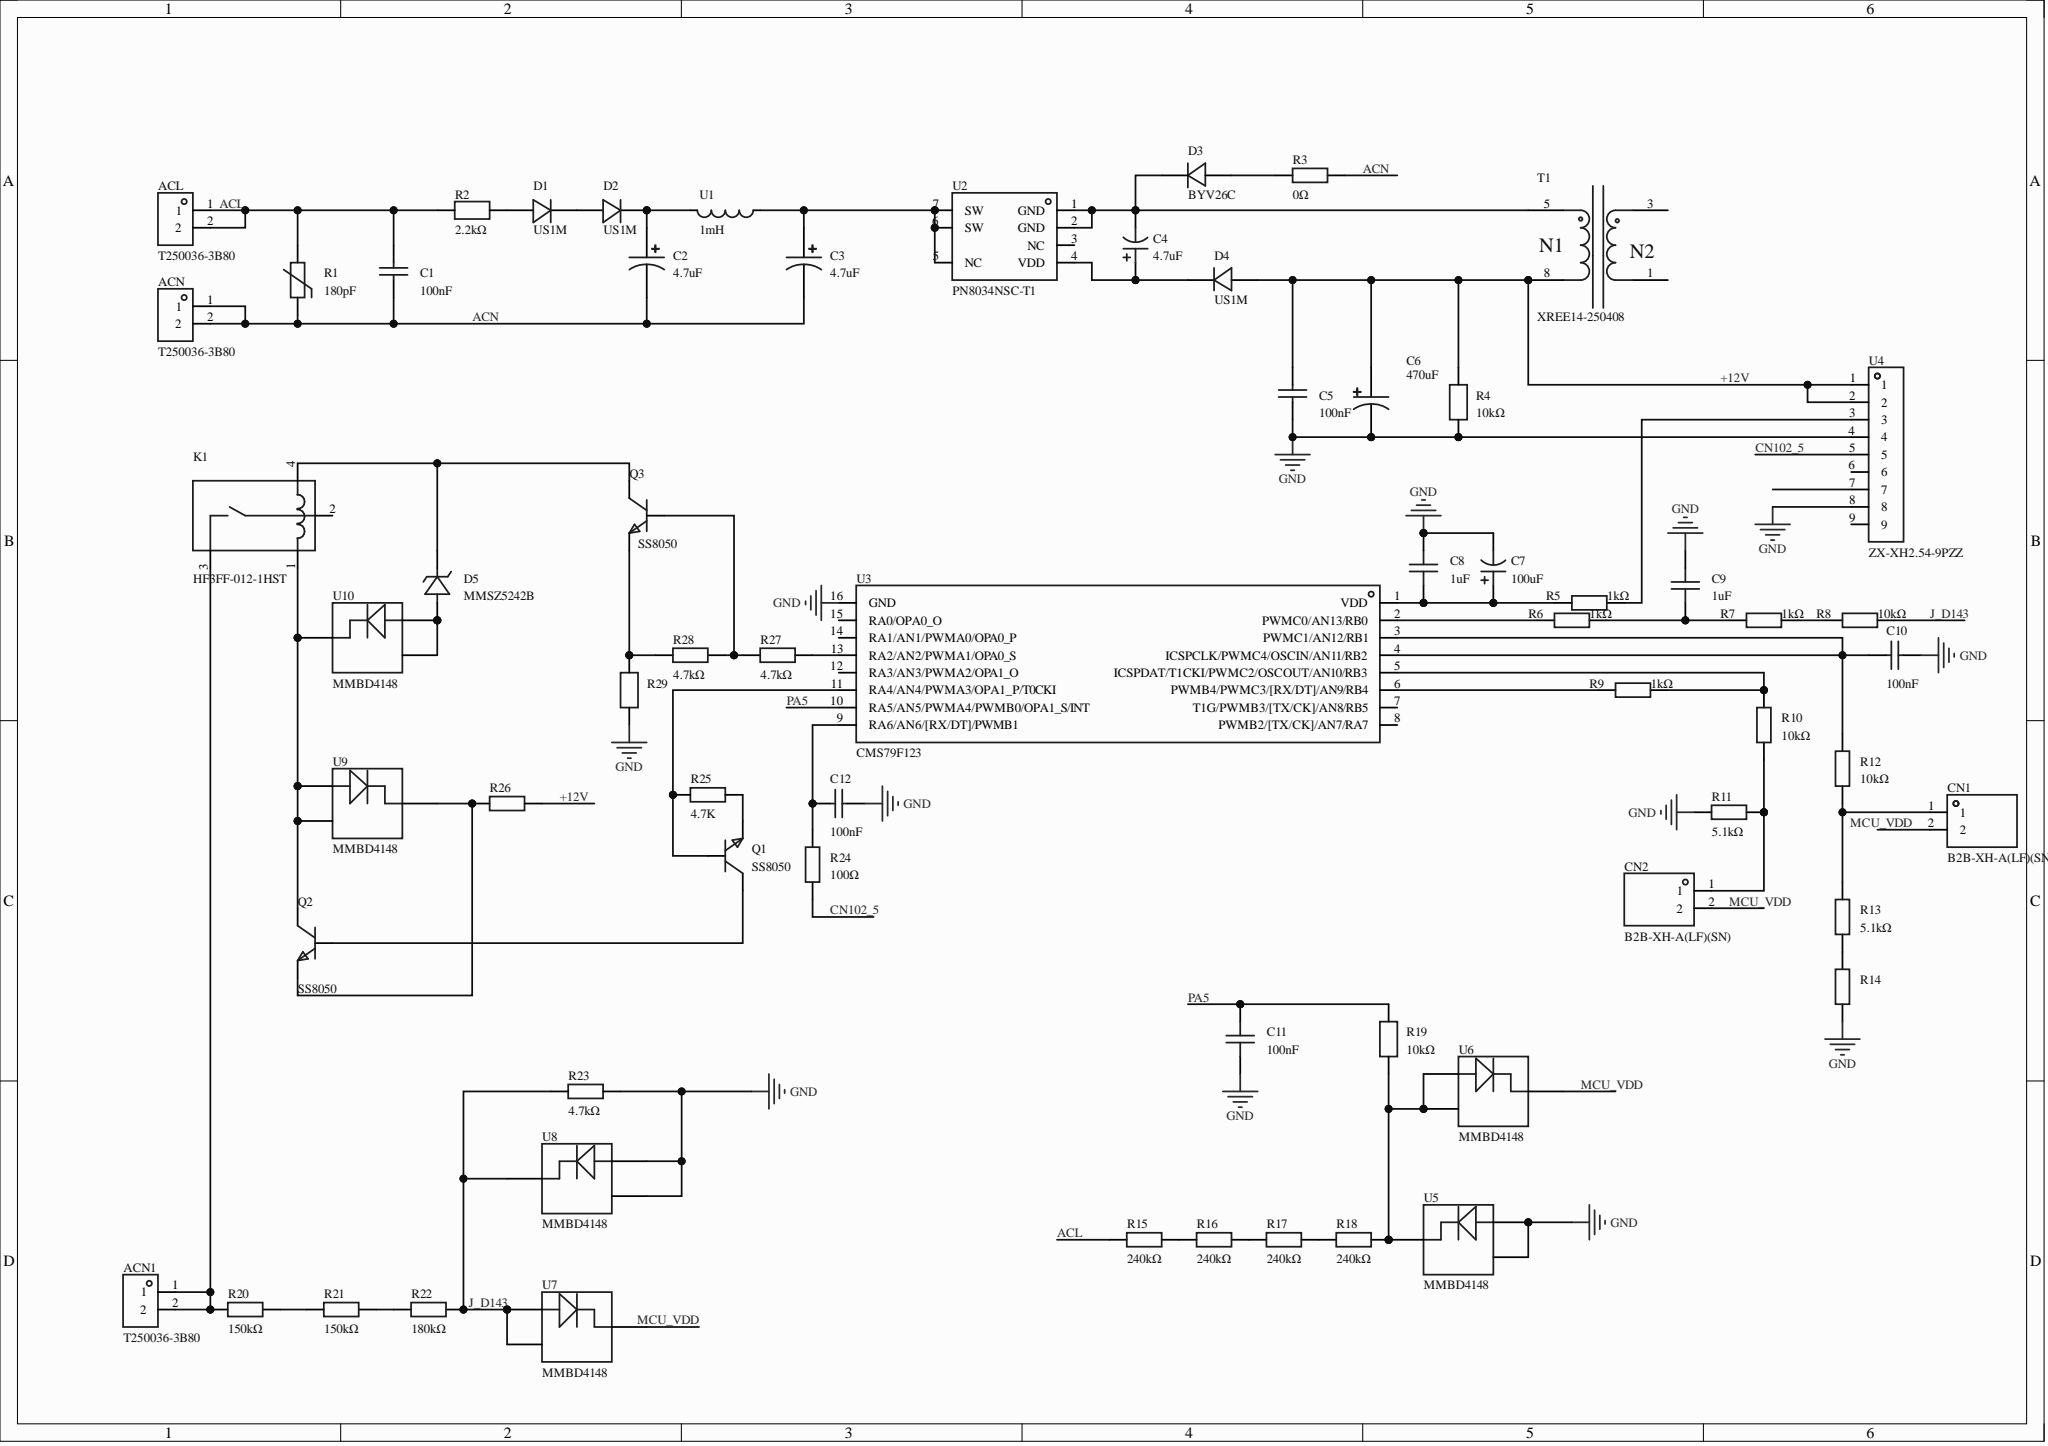Circuit board | Altium Designer | 66 parts | 44 nets
Bill of materials:
Comment,Description,Designator,Footprint,LibRef,Quantity
"T250036-3B80","250 tab terminal, two pins","ACL, ACN, ACN1","CONN-TH_XFCN-T250036-3B80","T250036-3B80","3"
"100nF","Capacitance:100nF;Tolerance:±10%;Working voltage(AC):275V;Safety class:X2;","C1","CAP-TH_L18.0-W6.0-P15.00-D1.2","MP2104K27D2X8LC","1"
"4.7uF","Capacitance:4.7uF;Tolerance:±20%;Rated voltage:450V;Ripple current:300mA@100kHz;Equivalent series resistance(ESR):3.5Ω@100kHz;","C2, C3","CAP-TH_BD10.0-P5.00-D1.0-FD","01EC1577SHG4.7uF450V","2"
"4.7uF","Capacitance:4.7uF;Tolerance:±20%;Rated voltage:50V;","C4","CAP-TH_BD6.3-P2.50-D0.5-FD","LKFC1101H4R7MF","1"
"100nF","Capacitance:100nF;Tolerance:±10%;Rated voltage:25V;Temperature coefficient:X7R;, [NoValue]","C5, C10, C11, C12","C0603","CL10B104KA8NNNC, CAP_0603","4"
"470uF","Capacitance:470uF;Tolerance:±20%;Rated voltage:25V;Ripple current:950mA@100kHz;","C6","CAP-TH_BD10.0-P5.00-D1.0-FD","RC025M471LO10*12TH-2A1E","1"
"100uF","Capacitance:100uF;Tolerance:±20%;Rated voltage:25V;","C7","CAP-TH_BD6.3-P2.50-D0.5-FD","ERG25V100M6X7","1"
"1uF","Capacitance:1uF;Tolerance:±10%;Rated voltage:25V;Temperature coefficient:X5R;","C8, C9","C0603","CGA0603X5R105K250JT","2"
"B2B-XH-A(LF)(SN)","","CN1, CN2","CONN-TH_B2B-XH-A-LF-SN","B2B-XH-A(LF)(SN)","2"
"US1M","Diode configuration:Single;Forward voltage(Vf):1.65V@1A;DC reverse voltage(Vr):1kV;Rectified current:1A;Reverse recovery time(Trr):75ns;","D1, D2, D4","SMA_L4.4-W2.8-LS5.4-RD","US1M_C412437","3"
"BYV26C","Diode configuration:Single;Forward voltage(Vf):2.5V@1A;DC reverse voltage(Vr):600V;Rectified current:1A;Reverse recovery time(Trr):30ns;","D3","SMA_L4.4-W2.6-LS5.1-FD","BYV26C_C2903924","1"
"MMSZ5242B","Diode configuration:Single;Zener voltage(nominal):12V;Zener voltage(range):11.4V~12.6V;Power dissipation(Pd):500mW;","D5","SOD-123_L2.7-W1.6-LS3.7-RD","MMSZ5242B_C19077426","1"
"HF3FF-012-1HST","Coil voltage:12V;Contact form:One normally open group:1A(SPST-NO);Contact rating(resistive load):10A@28VDC;10A@277VAC;Max switching voltage:277V@AC;28V@DC;Max switching current:15A;","K1","RELAY-TH_HF3FF-012-1HST","HF3FF-012-1HST","1"
"SS8050","[NoValue], Transistor type:NPN;Collector current(Ic):1.5A;Collector-emitter breakdown voltage(Vceo):25V;Power dissipation(Pd):300mW;DC current gain(hFE):120@100mA,1.0V;","Q1, Q2, Q3","SOT-23-3_L2.9-W1.3-P1.90-LS2.4-BR","SS8050, SS8050_C7420370","3"
"180pF","Varistor voltage:504V~616V;Clamping voltage:920V;Working voltage(DC):460V;Working voltage(AC):350V;","R1","RES-TH_L11.0-W5.5-P7.50-D0.8-S4.70","10D561K_C49072850","1"
"2.2kΩ","Resistor type:Metal film resistor;Resistance:2.2kΩ;Tolerance:±1%;Power:1W;Temperature coefficient:±200ppm/?;","R2","RES-TH_BD4.5-L11.5-P15.50-D0.8","MF1W-2.2KΩ±1%T","1"
"0Ω","Resistor type:Thick film resistor;Resistance:0Ω;Tolerance:±1%;Power:125mW;Working voltage:150V;Temperature coefficient:±800ppm/?;","R3","R0805","0805W8F0000T5E","1"
"10kΩ","Resistor type:Thick film resistor;Resistance:10kΩ;Tolerance:±1%;Power:100mW;Working voltage:75V;Temperature coefficient:±100ppm/?;, Resistor type:Thick film resistor;Resistance:1kΩ;Tolerance:±1%;Power:100mW;Working voltage:75V;Temperature coefficient:±100ppm/?;","R4, R8, R10, R12, R19, R29","R0603","FRC0603F1002TS, 0603WAF1001T5E","6"
"1kΩ","Resistor type:Thick film resistor;Resistance:1kΩ;Tolerance:±1%;Power:100mW;Working voltage:75V;Temperature coefficient:±100ppm/?;","R5, R6, R7, R9, R14","R0603","0603WAF1001T5E","5"
"5.1kΩ","Resistor type:Thick film resistor;Resistance:1kΩ;Tolerance:±1%;Power:100mW;Working voltage:75V;Temperature coefficient:±100ppm/?;","R11, R13","R0603","0603WAF1001T5E","2"
"240kΩ","Resistor type:Thick film resistor;Resistance:240kΩ;Tolerance:±1%;Power:125mW;Working voltage:150V;Temperature coefficient:±100ppm/?;","R15, R16, R17, R18","R0805","0805W8F2403T5E","4"
"150kΩ","Resistor type:Thick film resistor;Resistance:150kΩ;Tolerance:±1%;Power:125mW;Max working voltage:150V;Temperature coefficient:±100ppm/?;","R20, R21","R0805","0805W8F1503T5E","2"
"180kΩ","Resistor type:Thick film resistor;Resistance:180kΩ;Tolerance:±1%;Power:125mW;Max working voltage:150V;Temperature coefficient:±100ppm/?;","R22","R0805","0805W8F1803T5E","1"
"4.7kΩ","Resistor type:Metal film resistor;Resistance:4.7kΩ;Tolerance:±1%;Power:1W;Temperature coefficient:±50ppm/?;","R23","RES-TH_BD3.3-L9.0-P13.00-D0.6","RN1WS4.7KOFT/BA1","1"
"100Ω","Resistor type:Thick film resistor;Resistance:100Ω;Tolerance:±1%;Power:100mW;Max working voltage:75V;Temperature coefficient:±100ppm/?;","R24","R0603","RC0603FR-07100RL","1"
"4.7K","","R25, R26","R0603","Res_0603","2"
"4.7kΩ","Resistor type:Thick film resistor;Resistance:4.7kΩ;Tolerance:±1%;Power:100mW;Working voltage:75V;Temperature coefficient:±100ppm/?;","R27, R28","R0603","0603WAF4701T5E","2"
"XREE14-250408","Inductance:1.0mH@@Test condition:10KHZ 0.3V@@Withstand voltage test:P--C1000V/5mA/60S","T1","XFMR-TH_XREE14-250408","XREE14-250408","1"
"1mH","Inductance:1mH;Tolerance:±10%;Rated current:60mA;Saturation current(Isat):-;Type:Color-ring inductor;Q factor:60@0.796MHz;","U1","IND-TH_BD3.0-L8.0-P12.00-D0.6","YAL0307-102K","1"
"PN8034NSC-T1","Working voltage:10V~20V;Switching frequency:-;Output current:300mA;Transistor voltage rating:650V;","U2","DIP-8_7P-L9.3-W6.4-P2.54-LS7.6-BL-PE6","PN8034NSC-T1","1"
"CMS79F123","","U3","SOPN-16_L9.9-W3.9-P1.27-LS6.0-BL","CMS79F123","1"
"ZX-XH2.54-9PZZ","","U4","CONN-TH_9P-P2.50_ZX-XH2.54-9PZZ","ZX-XH2.54-9PZZ","1"
"MMBD4148","Forward voltage(Vf):1.25V@150mA;DC reverse voltage(Vr):75V;Rectified current:150mA;Reverse recovery time(Trr):4ns;","U5, U6, U7, U8, U9, U10","SOT-23-3_L2.9-W1.3-P1.90-LS2.4-BR","MMBD4148_C7461109","6"
Netlist (Protel format):
[
ACL
CONN-TH_XFCN-T250036-3B80
T250036-3B80



]
[
ACN
CONN-TH_XFCN-T250036-3B80
T250036-3B80



]
[
ACN1
CONN-TH_XFCN-T250036-3B80
T250036-3B80



]
[
C1
CAP-TH_L18.0-W6.0-P15.00-D1.2
100nF



]
[
C2
CAP-TH_BD10.0-P5.00-D1.0-FD
4.7uF



]
[
C3
CAP-TH_BD10.0-P5.00-D1.0-FD
4.7uF



]
[
C4
CAP-TH_BD6.3-P2.50-D0.5-FD
4.7uF



]
[
C5
C0603
100nF



]
[
C6
CAP-TH_BD10.0-P5.00-D1.0-FD
470uF



]
[
C7
CAP-TH_BD6.3-P2.50-D0.5-FD
100uF



]
[
C8
C0603
1uF



]
[
C9
C0603
1uF



]
[
C10
C0603
100nF



]
[
C11
C0603
100nF



]
[
C12
C0603
100nF



]
[
CN1
CONN-TH_B2B-XH-A-LF-SN
B2B-XH-A(LF)(SN)



]
[
CN2
CONN-TH_B2B-XH-A-LF-SN
B2B-XH-A(LF)(SN)



]
[
D1
SMA_L4.4-W2.8-LS5.4-RD
US1M



]
[
D2
SMA_L4.4-W2.8-LS5.4-RD
US1M



]
[
D3
SMA_L4.4-W2.6-LS5.1-FD
BYV26C



]
[
D4
SMA_L4.4-W2.8-LS5.4-RD
US1M



]
[
D5
SOD-123_L2.7-W1.6-LS3.7-RD
MMSZ5242B



]
[
K1
RELAY-TH_HF3FF-012-1HST
HF3FF-012-1HST



]
[
Q1
SOT-23-3_L2.9-W1.3-P1.90-LS2.4-BR
SS8050



]
[
Q2
SOT-23-3_L2.9-W1.3-P1.90-LS2.4-BR
SS8050



]
[
Q3
SOT-23-3_L2.9-W1.3-P1.90-LS2.4-BR
SS8050



]
[
R1
RES-TH_L11.0-W5.5-P7.50-D0.8-S4.70
180pF



]
[
R2
RES-TH_BD4.5-L11.5-P15.50-D0.8
2.2kΩ



]
[
R3
R0805
0Ω



]
[
R4
R0603
10kΩ



]
[
R5
R0603
1kΩ



]
[
R6
R0603
1kΩ



]
[
R7
R0603
1kΩ



]
[
R8
R0603
10kΩ



]
[
R9
R0603
1kΩ



]
[
R10
R0603
10kΩ



]
[
R11
R0603
5.1kΩ



]
[
R12
R0603
10kΩ



]
[
R13
R0603
5.1kΩ



]
[
R14
R0603
1kΩ



]
[
R15
R0805
240kΩ



]
[
R16
R0805
240kΩ



]
[
R17
R0805
240kΩ



]
[
R18
R0805
240kΩ



]
[
R19
R0603
10kΩ



]
[
R20
R0805
150kΩ



]
[
R21
R0805
150kΩ



]
[
R22
R0805
180kΩ



]
[
R23
RES-TH_BD3.3-L9.0-P13.00-D0.6
4.7kΩ



]
[
R24
R0603
100Ω



]
[
R25
R0603
4.7K



]
[
R26
R0603
4.7K



]
[
R27
R0603
4.7kΩ



]
[
R28
R0603
4.7kΩ



]
[
R29
R0603
10kΩ



]
[
T1
XFMR-TH_XREE14-250408
XREE14-250408



]
[
U1
IND-TH_BD3.0-L8.0-P12.00-D0.6
1mH



]
[
U2
DIP-8_7P-L9.3-W6.4-P2.54-LS7.6-BL-PE6
PN8034NSC-T1



]
[
U3
SOPN-16_L9.9-W3.9-P1.27-LS6.0-BL
CMS79F123



]
[
U4
CONN-TH_9P-P2.50_ZX-XH2.54-9PZZ
ZX-XH2.54-9PZZ



]
[
U5
SOT-23-3_L2.9-W1.3-P1.90-LS2.4-BR
MMBD4148



]
[
U6
SOT-23-3_L2.9-W1.3-P1.90-LS2.4-BR
MMBD4148



]
[
U7
SOT-23-3_L2.9-W1.3-P1.90-LS2.4-BR
MMBD4148



]
[
U8
SOT-23-3_L2.9-W1.3-P1.90-LS2.4-BR
MMBD4148



]
[
U9
SOT-23-3_L2.9-W1.3-P1.90-LS2.4-BR
MMBD4148



]
[
U10
SOT-23-3_L2.9-W1.3-P1.90-LS2.4-BR
MMBD4148



]
(
PA5
C11-2
R19-2
U3-10
)
(
NetR27_2
R27-2
U3-13
)
(
NetR21_2
R21-2
R22-1
)
(
NetR20_2
R20-2
R21-1
)
(
NetR18_2
R18-2
R19-1
U5-3
U6-1
U6-2
)
(
NetR17_2
R17-2
R18-1
)
(
NetR16_2
R16-2
R17-1
)
(
NetR15_2
R15-2
R16-1
)
(
NetR13_2
R13-2
R14-2
)
(
NetR9_2
R9-2
R10-2
U3-5
)
(
NetR9_1
R9-1
U3-6
)
(
NetR7_2
R7-2
R8-1
)
(
NetR6_1
R6-1
U3-2
)
(
NetR5_2
R5-2
U4-3
)
(
NetQ3_2
Q3-2
R28-1
R29-2
)
(
NetQ3_1
Q3-1
R27-1
R28-2
)
(
NetQ2_2
Q2-2
R26-1
U9-3
)
(
NetQ1_3
Q1-3
Q2-1
)
(
NetQ1_2
Q1-2
R25-2
)
(
NetQ1_1
Q1-1
R25-1
U3-11
)
(
NetK1_1
K1-1
Q2-3
U9-1
U9-2
U10-3
)
(
NetD5_2
D5-2
U10-1
U10-2
)
(
NetD5_1
D5-1
K1-4
Q3-3
)
(
NetD3_1
D3-1
R3-1
)
(
NetD1_2
D1-2
R2-2
)
(
NetD1_1
D1-1
D2-2
)
(
NetCN2_1
CN2-1
R10-1
R11-1
)
(
NetCN1_1
CN1-1
R12-1
R13-1
)
(
NetC12_1
C12-1
R24-2
U3-9
)
(
NetC10_2
C10-2
R12-2
U3-3
U3-4
)
(
NetC9_1
C9-1
R6-2
R7-1
)
(
NetC7_1
C7-1
C8-1
R5-1
U3-1
)
(
NetC4_2
C4-2
D3-2
T1-5
U2-1
U2-2
)
(
NetC4_1
C4-1
D4-1
U2-4
)
(
NetC3_1
C3-1
U1-2
U2-5
U2-6
U2-7
)
(
NetC2_1
C2-1
D2-1
U1-1
)
(
NetACN1_1
ACN1-1
ACN1-2
K1-3
R20-1
)
(
MCU_VDD
CN1-2
CN2-2
U6-3
U7-3
)
(
J_D143
R8-2
R22-2
R23-1
U7-1
U7-2
U8-3
)
(
GND
C5-1
C6-2
C7-2
C8-2
C9-2
C10-1
C11-1
C12-2
R4-1
R11-2
R14-1
R23-2
R29-1
U3-16
U4-4
U4-8
U5-1
U5-2
U8-1
U8-2
)
(
CN102_5
R24-1
U4-5
)
(
ACN
ACN-1
ACN-2
C1-1
C2-2
C3-2
R1-1
R3-2
)
(
ACL
ACL-1
ACL-2
C1-2
R1-2
R2-1
R15-1
)
(
+12V
C5-2
C6-1
D4-2
R4-2
R26-2
T1-8
U4-1
U4-2
)